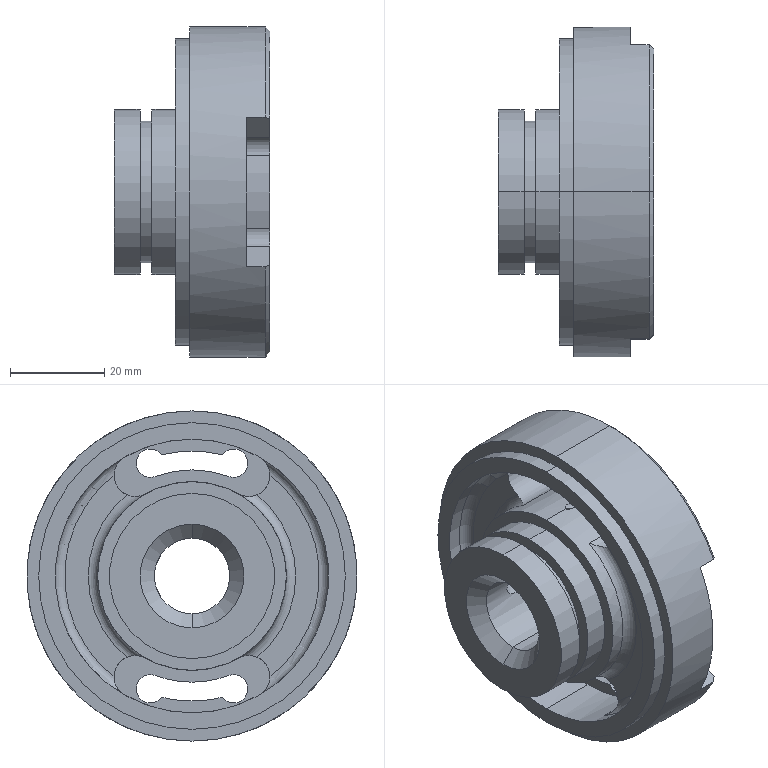Part | SolidWorks | features ICE 5, MirrorPattern 3, Chamfer 2, Fillet 2, 3DProfileFeature 1, HoleWzd 1, Revolution 1 | 1 solid | 96 faces | box 33 x 70 x 70 mm | volume 62726 mm3 | cylinder 60 | plane 19 | cone 13 | torus 4 | commonest cylinder face diameters 6 x16 45 x5 2 x4 3.3 x4 35 x4 9 x3